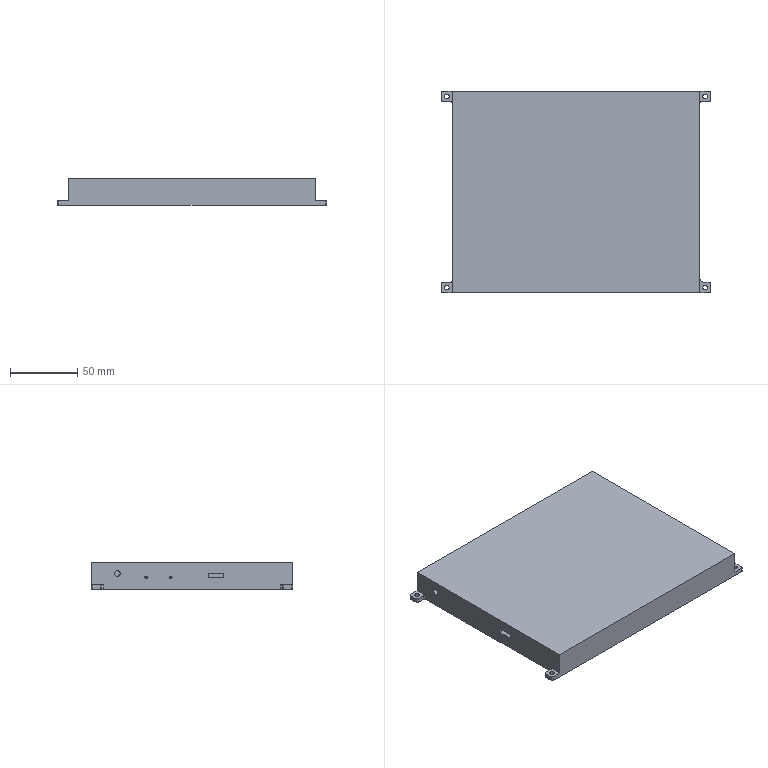Part | STEP file | SOLID | 1 solid | 49 faces | box 200 x 150 x 20 mm | volume 552493 mm3 | plane 25 | cylinder 20 | cone 4 | commonest cylinder face diameters 2 x11 3.5 x4 1.6 x2 4.1 x2 7 x1